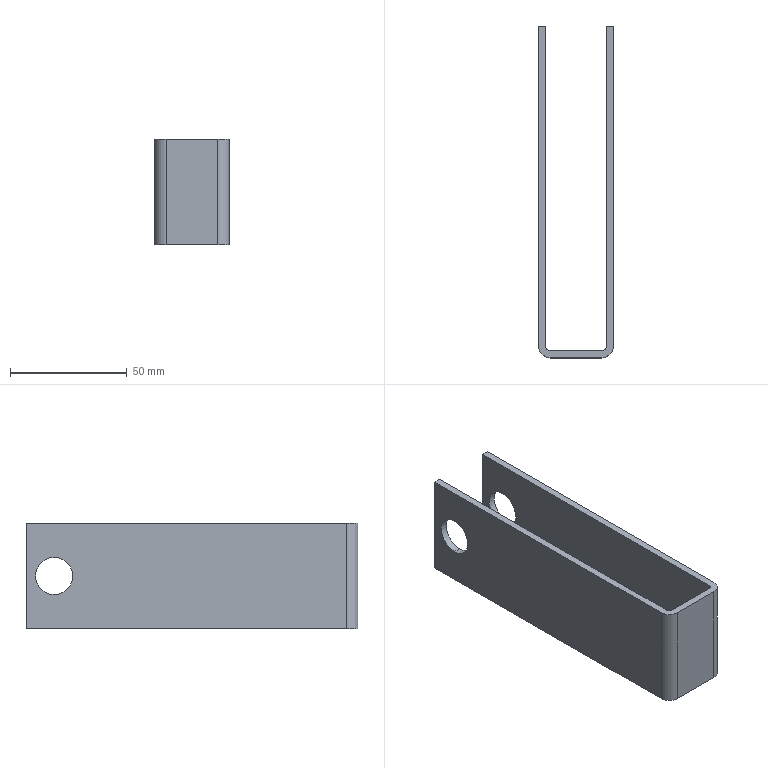Part | SolidWorks | features Extrusion 1, ICE 1 | 1 solid | 18 faces | box 32 x 142 x 45 mm | volume 40238 mm3 | plane 10 | cylinder 8 | commonest cylinder face diameters 16 x4 4 x2 10 x2
STEP:
#1=CARTESIAN_POINT('',(29.,-12.,30.5));
#2=VERTEX_POINT('',#1);
#3=CARTESIAN_POINT('',(29.,-12.,14.5));
#4=VERTEX_POINT('',#3);
#5=CARTESIAN_POINT('',(29.,-12.,22.5));
#6=DIRECTION('',(1.,0.,0.));
#7=DIRECTION('',(0.,1.,0.));
#8=AXIS2_PLACEMENT_3D('',#5,#6,#7);
#9=CIRCLE('',#8,8.);
#10=EDGE_CURVE('',#2,#4,#9,.T.);
#11=ORIENTED_EDGE('',*,*,#10,.F.);
#12=CARTESIAN_POINT('',(32.,-12.,30.5));
#13=VERTEX_POINT('',#12);
#14=CARTESIAN_POINT('',(0.,-12.,30.5));
#15=DIRECTION('',(1.,0.,0.));
#16=VECTOR('',#15,1000.);
#17=LINE('',#14,#16);
#18=EDGE_CURVE('',#2,#13,#17,.T.);
#19=ORIENTED_EDGE('',*,*,#18,.T.);
#20=CARTESIAN_POINT('',(32.,-12.,14.5));
#21=VERTEX_POINT('',#20);
#22=CARTESIAN_POINT('',(32.,-12.,22.5));
#23=DIRECTION('',(1.,0.,0.));
#24=DIRECTION('',(0.,0.,-1.));
#25=AXIS2_PLACEMENT_3D('',#22,#23,#24);
#26=CIRCLE('',#25,8.);
#27=EDGE_CURVE('',#13,#21,#26,.T.);
#28=ORIENTED_EDGE('',*,*,#27,.T.);
#29=CARTESIAN_POINT('',(0.,-12.,14.5));
#30=DIRECTION('',(1.,0.,0.));
#31=VECTOR('',#30,1000.);
#32=LINE('',#29,#31);
#33=EDGE_CURVE('',#4,#21,#32,.T.);
#34=ORIENTED_EDGE('',*,*,#33,.F.);
#35=EDGE_LOOP('',(#11,#19,#28,#34));
#36=FACE_OUTER_BOUND('',#35,.T.);
#37=CARTESIAN_POINT('',(0.,-12.,22.5));
#38=DIRECTION('',(1.,0.,0.));
#39=DIRECTION('',(0.,0.,-1.));
#40=AXIS2_PLACEMENT_3D('',#37,#38,#39);
#41=CYLINDRICAL_SURFACE('',#40,8.);
#42=ADVANCED_FACE('',(#36),#41,.F.);
#43=CARTESIAN_POINT('',(0.,-12.,30.5));
#44=VERTEX_POINT('',#43);
#45=CARTESIAN_POINT('',(0.,-12.,14.5));
#46=VERTEX_POINT('',#45);
#47=CARTESIAN_POINT('',(0.,-12.,22.5));
#48=DIRECTION('',(1.,0.,0.));
#49=DIRECTION('',(0.,0.,-1.));
#50=AXIS2_PLACEMENT_3D('',#47,#48,#49);
#51=CIRCLE('',#50,8.);
#52=EDGE_CURVE('',#44,#46,#51,.T.);
#53=ORIENTED_EDGE('',*,*,#52,.F.);
#54=CARTESIAN_POINT('',(3.,-12.,30.5));
#55=VERTEX_POINT('',#54);
#56=CARTESIAN_POINT('',(0.,-12.,30.5));
#57=DIRECTION('',(1.,0.,0.));
#58=VECTOR('',#57,1000.);
#59=LINE('',#56,#58);
#60=EDGE_CURVE('',#44,#55,#59,.T.);
#61=ORIENTED_EDGE('',*,*,#60,.T.);
#62=CARTESIAN_POINT('',(3.,-12.,14.5));
#63=VERTEX_POINT('',#62);
#64=CARTESIAN_POINT('',(3.,-12.,22.5));
#65=DIRECTION('',(-1.,0.,0.));
#66=DIRECTION('',(0.,-1.,0.));
#67=AXIS2_PLACEMENT_3D('',#64,#65,#66);
#68=CIRCLE('',#67,8.);
#69=EDGE_CURVE('',#63,#55,#68,.T.);
#70=ORIENTED_EDGE('',*,*,#69,.F.);
#71=CARTESIAN_POINT('',(0.,-12.,14.5));
#72=DIRECTION('',(1.,0.,0.));
#73=VECTOR('',#72,1000.);
#74=LINE('',#71,#73);
#75=EDGE_CURVE('',#46,#63,#74,.T.);
#76=ORIENTED_EDGE('',*,*,#75,.F.);
#77=EDGE_LOOP('',(#53,#61,#70,#76));
#78=FACE_OUTER_BOUND('',#77,.T.);
#79=CARTESIAN_POINT('',(0.,-12.,22.5));
#80=DIRECTION('',(1.,0.,0.));
#81=DIRECTION('',(0.,0.,-1.));
#82=AXIS2_PLACEMENT_3D('',#79,#80,#81);
#83=CYLINDRICAL_SURFACE('',#82,8.);
#84=ADVANCED_FACE('',(#78),#83,.F.);
#85=CARTESIAN_POINT('',(3.,0.,0.));
#86=VERTEX_POINT('',#85);
#87=CARTESIAN_POINT('',(0.,0.,0.));
#88=VERTEX_POINT('',#87);
#89=CARTESIAN_POINT('',(3.,0.,0.));
#90=DIRECTION('',(-1.,0.,0.));
#91=VECTOR('',#90,1000.);
#92=LINE('',#89,#91);
#93=EDGE_CURVE('',#86,#88,#92,.T.);
#94=ORIENTED_EDGE('',*,*,#93,.T.);
#95=CARTESIAN_POINT('',(0.,0.,45.));
#96=VERTEX_POINT('',#95);
#97=CARTESIAN_POINT('',(0.,0.,45.));
#98=DIRECTION('',(0.,0.,-1.));
#99=VECTOR('',#98,1000.);
#100=LINE('',#97,#99);
#101=EDGE_CURVE('',#96,#88,#100,.T.);
#102=ORIENTED_EDGE('',*,*,#101,.F.);
#103=CARTESIAN_POINT('',(3.,0.,45.));
#104=VERTEX_POINT('',#103);
#105=CARTESIAN_POINT('',(3.,0.,45.));
#106=DIRECTION('',(-1.,0.,0.));
#107=VECTOR('',#106,1000.);
#108=LINE('',#105,#107);
#109=EDGE_CURVE('',#104,#96,#108,.T.);
#110=ORIENTED_EDGE('',*,*,#109,.F.);
#111=CARTESIAN_POINT('',(3.,0.,45.));
#112=DIRECTION('',(0.,0.,-1.));
#113=VECTOR('',#112,1000.);
#114=LINE('',#111,#113);
#115=EDGE_CURVE('',#104,#86,#114,.T.);
#116=ORIENTED_EDGE('',*,*,#115,.T.);
#117=EDGE_LOOP('',(#94,#102,#110,#116));
#118=FACE_OUTER_BOUND('',#117,.T.);
#119=CARTESIAN_POINT('',(3.,0.,45.));
#120=DIRECTION('',(0.,-1.,0.));
#121=DIRECTION('',(0.,0.,-1.));
#122=AXIS2_PLACEMENT_3D('',#119,#120,#121);
#123=PLANE('',#122);
#124=ADVANCED_FACE('',(#118),#123,.F.);
#125=CARTESIAN_POINT('',(0.,-12.,22.5));
#126=DIRECTION('',(1.,0.,0.));
#127=DIRECTION('',(0.,0.,-1.));
#128=AXIS2_PLACEMENT_3D('',#125,#126,#127);
#129=CIRCLE('',#128,8.);
#130=EDGE_CURVE('',#46,#44,#129,.T.);
#131=ORIENTED_EDGE('',*,*,#130,.T.);
#132=ORIENTED_EDGE('',*,*,#52,.T.);
#133=EDGE_LOOP('',(#131,#132));
#134=FACE_BOUND('',#133,.T.);
#135=CARTESIAN_POINT('',(0.,-137.,0.));
#136=VERTEX_POINT('',#135);
#137=CARTESIAN_POINT('',(0.,0.,0.));
#138=DIRECTION('',(0.,-1.,0.));
#139=VECTOR('',#138,1000.);
#140=LINE('',#137,#139);
#141=EDGE_CURVE('',#88,#136,#140,.T.);
#142=ORIENTED_EDGE('',*,*,#141,.T.);
#143=CARTESIAN_POINT('',(0.,-137.,45.));
#144=VERTEX_POINT('',#143);
#145=CARTESIAN_POINT('',(0.,-137.,45.));
#146=DIRECTION('',(0.,0.,-1.));
#147=VECTOR('',#146,1000.);
#148=LINE('',#145,#147);
#149=EDGE_CURVE('',#144,#136,#148,.T.);
#150=ORIENTED_EDGE('',*,*,#149,.F.);
#151=CARTESIAN_POINT('',(0.,0.,45.));
#152=DIRECTION('',(0.,-1.,0.));
#153=VECTOR('',#152,1000.);
#154=LINE('',#151,#153);
#155=EDGE_CURVE('',#96,#144,#154,.T.);
#156=ORIENTED_EDGE('',*,*,#155,.F.);
#157=ORIENTED_EDGE('',*,*,#101,.T.);
#158=EDGE_LOOP('',(#142,#150,#156,#157));
#159=FACE_OUTER_BOUND('',#158,.T.);
#160=CARTESIAN_POINT('',(0.,0.,45.));
#161=DIRECTION('',(1.,0.,0.));
#162=DIRECTION('',(0.,1.,0.));
#163=AXIS2_PLACEMENT_3D('',#160,#161,#162);
#164=PLANE('',#163);
#165=ADVANCED_FACE('',(#134,#159),#164,.F.);
#166=CARTESIAN_POINT('',(5.,-142.,0.));
#167=VERTEX_POINT('',#166);
#168=CARTESIAN_POINT('',(5.,-137.,0.));
#169=DIRECTION('',(0.,0.,1.));
#170=DIRECTION('',(1.,0.,0.));
#171=AXIS2_PLACEMENT_3D('',#168,#169,#170);
#172=CIRCLE('',#171,5.);
#173=EDGE_CURVE('',#136,#167,#172,.T.);
#174=ORIENTED_EDGE('',*,*,#173,.T.);
#175=CARTESIAN_POINT('',(5.,-142.,45.));
#176=VERTEX_POINT('',#175);
#177=CARTESIAN_POINT('',(5.,-142.,45.));
#178=DIRECTION('',(0.,0.,-1.));
#179=VECTOR('',#178,1000.);
#180=LINE('',#177,#179);
#181=EDGE_CURVE('',#176,#167,#180,.T.);
#182=ORIENTED_EDGE('',*,*,#181,.F.);
#183=CARTESIAN_POINT('',(5.,-137.,45.));
#184=DIRECTION('',(0.,0.,1.));
#185=DIRECTION('',(1.,0.,0.));
#186=AXIS2_PLACEMENT_3D('',#183,#184,#185);
#187=CIRCLE('',#186,5.);
#188=EDGE_CURVE('',#144,#176,#187,.T.);
#189=ORIENTED_EDGE('',*,*,#188,.F.);
#190=ORIENTED_EDGE('',*,*,#149,.T.);
#191=EDGE_LOOP('',(#174,#182,#189,#190));
#192=FACE_OUTER_BOUND('',#191,.T.);
#193=CARTESIAN_POINT('',(5.,-137.,45.));
#194=DIRECTION('',(0.,0.,-1.));
#195=DIRECTION('',(-1.,0.,0.));
#196=AXIS2_PLACEMENT_3D('',#193,#194,#195);
#197=CYLINDRICAL_SURFACE('',#196,5.);
#198=ADVANCED_FACE('',(#192),#197,.T.);
#199=CARTESIAN_POINT('',(27.,-142.,0.));
#200=VERTEX_POINT('',#199);
#201=CARTESIAN_POINT('',(5.,-142.,0.));
#202=DIRECTION('',(1.,0.,0.));
#203=VECTOR('',#202,1000.);
#204=LINE('',#201,#203);
#205=EDGE_CURVE('',#167,#200,#204,.T.);
#206=ORIENTED_EDGE('',*,*,#205,.T.);
#207=CARTESIAN_POINT('',(27.,-142.,45.));
#208=VERTEX_POINT('',#207);
#209=CARTESIAN_POINT('',(27.,-142.,45.));
#210=DIRECTION('',(0.,0.,-1.));
#211=VECTOR('',#210,1000.);
#212=LINE('',#209,#211);
#213=EDGE_CURVE('',#208,#200,#212,.T.);
#214=ORIENTED_EDGE('',*,*,#213,.F.);
#215=CARTESIAN_POINT('',(5.,-142.,45.));
#216=DIRECTION('',(1.,0.,0.));
#217=VECTOR('',#216,1000.);
#218=LINE('',#215,#217);
#219=EDGE_CURVE('',#176,#208,#218,.T.);
#220=ORIENTED_EDGE('',*,*,#219,.F.);
#221=ORIENTED_EDGE('',*,*,#181,.T.);
#222=EDGE_LOOP('',(#206,#214,#220,#221));
#223=FACE_OUTER_BOUND('',#222,.T.);
#224=CARTESIAN_POINT('',(5.,-142.,45.));
#225=DIRECTION('',(0.,1.,0.));
#226=DIRECTION('',(0.,0.,1.));
#227=AXIS2_PLACEMENT_3D('',#224,#225,#226);
#228=PLANE('',#227);
#229=ADVANCED_FACE('',(#223),#228,.F.);
#230=CARTESIAN_POINT('',(32.,-137.,0.));
#231=VERTEX_POINT('',#230);
#232=CARTESIAN_POINT('',(27.,-137.,0.));
#233=DIRECTION('',(0.,0.,1.));
#234=DIRECTION('',(1.,0.,0.));
#235=AXIS2_PLACEMENT_3D('',#232,#233,#234);
#236=CIRCLE('',#235,5.);
#237=EDGE_CURVE('',#200,#231,#236,.T.);
#238=ORIENTED_EDGE('',*,*,#237,.T.);
#239=CARTESIAN_POINT('',(32.,-137.,45.));
#240=VERTEX_POINT('',#239);
#241=CARTESIAN_POINT('',(32.,-137.,45.));
#242=DIRECTION('',(0.,0.,-1.));
#243=VECTOR('',#242,1000.);
#244=LINE('',#241,#243);
#245=EDGE_CURVE('',#240,#231,#244,.T.);
#246=ORIENTED_EDGE('',*,*,#245,.F.);
#247=CARTESIAN_POINT('',(27.,-137.,45.));
#248=DIRECTION('',(0.,0.,1.));
#249=DIRECTION('',(1.,0.,0.));
#250=AXIS2_PLACEMENT_3D('',#247,#248,#249);
#251=CIRCLE('',#250,5.);
#252=EDGE_CURVE('',#208,#240,#251,.T.);
#253=ORIENTED_EDGE('',*,*,#252,.F.);
#254=ORIENTED_EDGE('',*,*,#213,.T.);
#255=EDGE_LOOP('',(#238,#246,#253,#254));
#256=FACE_OUTER_BOUND('',#255,.T.);
#257=CARTESIAN_POINT('',(27.,-137.,45.));
#258=DIRECTION('',(0.,0.,-1.));
#259=DIRECTION('',(-1.,0.,0.));
#260=AXIS2_PLACEMENT_3D('',#257,#258,#259);
#261=CYLINDRICAL_SURFACE('',#260,5.);
#262=ADVANCED_FACE('',(#256),#261,.T.);
#263=CARTESIAN_POINT('',(32.,-12.,22.5));
#264=DIRECTION('',(1.,0.,0.));
#265=DIRECTION('',(0.,0.,-1.));
#266=AXIS2_PLACEMENT_3D('',#263,#264,#265);
#267=CIRCLE('',#266,8.);
#268=EDGE_CURVE('',#21,#13,#267,.T.);
#269=ORIENTED_EDGE('',*,*,#268,.F.);
#270=ORIENTED_EDGE('',*,*,#27,.F.);
#271=EDGE_LOOP('',(#269,#270));
#272=FACE_BOUND('',#271,.T.);
#273=CARTESIAN_POINT('',(32.,0.,0.));
#274=VERTEX_POINT('',#273);
#275=CARTESIAN_POINT('',(32.,-137.,0.));
#276=DIRECTION('',(0.,1.,0.));
#277=VECTOR('',#276,1000.);
#278=LINE('',#275,#277);
#279=EDGE_CURVE('',#231,#274,#278,.T.);
#280=ORIENTED_EDGE('',*,*,#279,.T.);
#281=CARTESIAN_POINT('',(32.,0.,45.));
#282=VERTEX_POINT('',#281);
#283=CARTESIAN_POINT('',(32.,0.,45.));
#284=DIRECTION('',(0.,0.,-1.));
#285=VECTOR('',#284,1000.);
#286=LINE('',#283,#285);
#287=EDGE_CURVE('',#282,#274,#286,.T.);
#288=ORIENTED_EDGE('',*,*,#287,.F.);
#289=CARTESIAN_POINT('',(32.,-137.,45.));
#290=DIRECTION('',(0.,1.,0.));
#291=VECTOR('',#290,1000.);
#292=LINE('',#289,#291);
#293=EDGE_CURVE('',#240,#282,#292,.T.);
#294=ORIENTED_EDGE('',*,*,#293,.F.);
#295=ORIENTED_EDGE('',*,*,#245,.T.);
#296=EDGE_LOOP('',(#280,#288,#294,#295));
#297=FACE_OUTER_BOUND('',#296,.T.);
#298=CARTESIAN_POINT('',(32.,-137.,45.));
#299=DIRECTION('',(-1.,0.,0.));
#300=DIRECTION('',(0.,-1.,0.));
#301=AXIS2_PLACEMENT_3D('',#298,#299,#300);
#302=PLANE('',#301);
#303=ADVANCED_FACE('',(#272,#297),#302,.F.);
#304=CARTESIAN_POINT('',(29.,0.,0.));
#305=VERTEX_POINT('',#304);
#306=CARTESIAN_POINT('',(29.,0.,0.));
#307=DIRECTION('',(-1.,0.,0.));
#308=VECTOR('',#307,1000.);
#309=LINE('',#306,#308);
#310=EDGE_CURVE('',#274,#305,#309,.T.);
#311=ORIENTED_EDGE('',*,*,#310,.T.);
#312=CARTESIAN_POINT('',(29.,0.,45.));
#313=VERTEX_POINT('',#312);
#314=CARTESIAN_POINT('',(29.,0.,45.));
#315=DIRECTION('',(0.,0.,-1.));
#316=VECTOR('',#315,1000.);
#317=LINE('',#314,#316);
#318=EDGE_CURVE('',#313,#305,#317,.T.);
#319=ORIENTED_EDGE('',*,*,#318,.F.);
#320=CARTESIAN_POINT('',(29.,0.,45.));
#321=DIRECTION('',(-1.,0.,0.));
#322=VECTOR('',#321,1000.);
#323=LINE('',#320,#322);
#324=EDGE_CURVE('',#282,#313,#323,.T.);
#325=ORIENTED_EDGE('',*,*,#324,.F.);
#326=ORIENTED_EDGE('',*,*,#287,.T.);
#327=EDGE_LOOP('',(#311,#319,#325,#326));
#328=FACE_OUTER_BOUND('',#327,.T.);
#329=CARTESIAN_POINT('',(29.,0.,45.));
#330=DIRECTION('',(0.,-1.,0.));
#331=DIRECTION('',(1.,0.,0.));
#332=AXIS2_PLACEMENT_3D('',#329,#330,#331);
#333=PLANE('',#332);
#334=ADVANCED_FACE('',(#328),#333,.F.);
#335=CARTESIAN_POINT('',(29.,-12.,22.5));
#336=DIRECTION('',(1.,0.,0.));
#337=DIRECTION('',(0.,1.,0.));
#338=AXIS2_PLACEMENT_3D('',#335,#336,#337);
#339=CIRCLE('',#338,8.);
#340=EDGE_CURVE('',#4,#2,#339,.T.);
#341=ORIENTED_EDGE('',*,*,#340,.T.);
#342=ORIENTED_EDGE('',*,*,#10,.T.);
#343=EDGE_LOOP('',(#341,#342));
#344=FACE_BOUND('',#343,.T.);
#345=CARTESIAN_POINT('',(29.,-137.,0.));
#346=VERTEX_POINT('',#345);
#347=CARTESIAN_POINT('',(29.,-137.,0.));
#348=DIRECTION('',(0.,-1.,0.));
#349=VECTOR('',#348,1000.);
#350=LINE('',#347,#349);
#351=EDGE_CURVE('',#305,#346,#350,.T.);
#352=ORIENTED_EDGE('',*,*,#351,.T.);
#353=CARTESIAN_POINT('',(29.,-137.,45.));
#354=VERTEX_POINT('',#353);
#355=CARTESIAN_POINT('',(29.,-137.,45.));
#356=DIRECTION('',(0.,0.,-1.));
#357=VECTOR('',#356,1000.);
#358=LINE('',#355,#357);
#359=EDGE_CURVE('',#354,#346,#358,.T.);
#360=ORIENTED_EDGE('',*,*,#359,.F.);
#361=CARTESIAN_POINT('',(29.,-137.,45.));
#362=DIRECTION('',(0.,-1.,0.));
#363=VECTOR('',#362,1000.);
#364=LINE('',#361,#363);
#365=EDGE_CURVE('',#313,#354,#364,.T.);
#366=ORIENTED_EDGE('',*,*,#365,.F.);
#367=ORIENTED_EDGE('',*,*,#318,.T.);
#368=EDGE_LOOP('',(#352,#360,#366,#367));
#369=FACE_OUTER_BOUND('',#368,.T.);
#370=CARTESIAN_POINT('',(29.,-137.,45.));
#371=DIRECTION('',(1.,0.,0.));
#372=DIRECTION('',(0.,1.,0.));
#373=AXIS2_PLACEMENT_3D('',#370,#371,#372);
#374=PLANE('',#373);
#375=ADVANCED_FACE('',(#344,#369),#374,.F.);
#376=CARTESIAN_POINT('',(27.,-139.,0.));
#377=VERTEX_POINT('',#376);
#378=CARTESIAN_POINT('',(27.,-137.,0.));
#379=DIRECTION('',(0.,0.,-1.));
#380=DIRECTION('',(1.,0.,0.));
#381=AXIS2_PLACEMENT_3D('',#378,#379,#380);
#382=CIRCLE('',#381,2.);
#383=EDGE_CURVE('',#346,#377,#382,.T.);
#384=ORIENTED_EDGE('',*,*,#383,.T.);
#385=CARTESIAN_POINT('',(27.,-139.,45.));
#386=VERTEX_POINT('',#385);
#387=CARTESIAN_POINT('',(27.,-139.,45.));
#388=DIRECTION('',(0.,0.,-1.));
#389=VECTOR('',#388,1000.);
#390=LINE('',#387,#389);
#391=EDGE_CURVE('',#386,#377,#390,.T.);
#392=ORIENTED_EDGE('',*,*,#391,.F.);
#393=CARTESIAN_POINT('',(27.,-137.,45.));
#394=DIRECTION('',(0.,0.,-1.));
#395=DIRECTION('',(1.,0.,0.));
#396=AXIS2_PLACEMENT_3D('',#393,#394,#395);
#397=CIRCLE('',#396,2.);
#398=EDGE_CURVE('',#354,#386,#397,.T.);
#399=ORIENTED_EDGE('',*,*,#398,.F.);
#400=ORIENTED_EDGE('',*,*,#359,.T.);
#401=EDGE_LOOP('',(#384,#392,#399,#400));
#402=FACE_OUTER_BOUND('',#401,.T.);
#403=CARTESIAN_POINT('',(27.,-137.,45.));
#404=DIRECTION('',(0.,0.,-1.));
#405=DIRECTION('',(-1.,0.,0.));
#406=AXIS2_PLACEMENT_3D('',#403,#404,#405);
#407=CYLINDRICAL_SURFACE('',#406,2.);
#408=ADVANCED_FACE('',(#402),#407,.F.);
#409=CARTESIAN_POINT('',(5.,-139.,0.));
#410=VERTEX_POINT('',#409);
#411=CARTESIAN_POINT('',(5.,-139.,0.));
#412=DIRECTION('',(-1.,0.,0.));
#413=VECTOR('',#412,1000.);
#414=LINE('',#411,#413);
#415=EDGE_CURVE('',#377,#410,#414,.T.);
#416=ORIENTED_EDGE('',*,*,#415,.T.);
#417=CARTESIAN_POINT('',(5.,-139.,45.));
#418=VERTEX_POINT('',#417);
#419=CARTESIAN_POINT('',(5.,-139.,45.));
#420=DIRECTION('',(0.,0.,-1.));
#421=VECTOR('',#420,1000.);
#422=LINE('',#419,#421);
#423=EDGE_CURVE('',#418,#410,#422,.T.);
#424=ORIENTED_EDGE('',*,*,#423,.F.);
#425=CARTESIAN_POINT('',(5.,-139.,45.));
#426=DIRECTION('',(-1.,0.,0.));
#427=VECTOR('',#426,1000.);
#428=LINE('',#425,#427);
#429=EDGE_CURVE('',#386,#418,#428,.T.);
#430=ORIENTED_EDGE('',*,*,#429,.F.);
#431=ORIENTED_EDGE('',*,*,#391,.T.);
#432=EDGE_LOOP('',(#416,#424,#430,#431));
#433=FACE_OUTER_BOUND('',#432,.T.);
#434=CARTESIAN_POINT('',(5.,-139.,45.));
#435=DIRECTION('',(0.,-1.,0.));
#436=DIRECTION('',(0.,0.,-1.));
#437=AXIS2_PLACEMENT_3D('',#434,#435,#436);
#438=PLANE('',#437);
#439=ADVANCED_FACE('',(#433),#438,.F.);
#440=CARTESIAN_POINT('',(3.,-137.,0.));
#441=VERTEX_POINT('',#440);
#442=CARTESIAN_POINT('',(5.,-137.,0.));
#443=DIRECTION('',(0.,0.,-1.));
#444=DIRECTION('',(1.,0.,0.));
#445=AXIS2_PLACEMENT_3D('',#442,#443,#444);
#446=CIRCLE('',#445,2.);
#447=EDGE_CURVE('',#410,#441,#446,.T.);
#448=ORIENTED_EDGE('',*,*,#447,.T.);
#449=CARTESIAN_POINT('',(3.,-137.,45.));
#450=VERTEX_POINT('',#449);
#451=CARTESIAN_POINT('',(3.,-137.,45.));
#452=DIRECTION('',(0.,0.,-1.));
#453=VECTOR('',#452,1000.);
#454=LINE('',#451,#453);
#455=EDGE_CURVE('',#450,#441,#454,.T.);
#456=ORIENTED_EDGE('',*,*,#455,.F.);
#457=CARTESIAN_POINT('',(5.,-137.,45.));
#458=DIRECTION('',(0.,0.,-1.));
#459=DIRECTION('',(1.,0.,0.));
#460=AXIS2_PLACEMENT_3D('',#457,#458,#459);
#461=CIRCLE('',#460,2.);
#462=EDGE_CURVE('',#418,#450,#461,.T.);
#463=ORIENTED_EDGE('',*,*,#462,.F.);
#464=ORIENTED_EDGE('',*,*,#423,.T.);
#465=EDGE_LOOP('',(#448,#456,#463,#464));
#466=FACE_OUTER_BOUND('',#465,.T.);
#467=CARTESIAN_POINT('',(5.,-137.,45.));
#468=DIRECTION('',(0.,0.,-1.));
#469=DIRECTION('',(-1.,0.,0.));
#470=AXIS2_PLACEMENT_3D('',#467,#468,#469);
#471=CYLINDRICAL_SURFACE('',#470,2.);
#472=ADVANCED_FACE('',(#466),#471,.F.);
#473=ORIENTED_EDGE('',*,*,#69,.T.);
#474=CARTESIAN_POINT('',(3.,-12.,22.5));
#475=DIRECTION('',(-1.,0.,0.));
#476=DIRECTION('',(0.,-1.,0.));
#477=AXIS2_PLACEMENT_3D('',#474,#475,#476);
#478=CIRCLE('',#477,8.);
#479=EDGE_CURVE('',#55,#63,#478,.T.);
#480=ORIENTED_EDGE('',*,*,#479,.T.);
#481=EDGE_LOOP('',(#473,#480));
#482=FACE_BOUND('',#481,.T.);
#483=CARTESIAN_POINT('',(3.,0.,0.));
#484=DIRECTION('',(0.,1.,0.));
#485=VECTOR('',#484,1000.);
#486=LINE('',#483,#485);
#487=EDGE_CURVE('',#441,#86,#486,.T.);
#488=ORIENTED_EDGE('',*,*,#487,.T.);
#489=ORIENTED_EDGE('',*,*,#115,.F.);
#490=CARTESIAN_POINT('',(3.,0.,45.));
#491=DIRECTION('',(0.,1.,0.));
#492=VECTOR('',#491,1000.);
#493=LINE('',#490,#492);
#494=EDGE_CURVE('',#450,#104,#493,.T.);
#495=ORIENTED_EDGE('',*,*,#494,.F.);
#496=ORIENTED_EDGE('',*,*,#455,.T.);
#497=EDGE_LOOP('',(#488,#489,#495,#496));
#498=FACE_OUTER_BOUND('',#497,.T.);
#499=CARTESIAN_POINT('',(3.,0.,45.));
#500=DIRECTION('',(-1.,0.,0.));
#501=DIRECTION('',(0.,-1.,0.));
#502=AXIS2_PLACEMENT_3D('',#499,#500,#501);
#503=PLANE('',#502);
#504=ADVANCED_FACE('',(#482,#498),#503,.F.);
#505=ORIENTED_EDGE('',*,*,#109,.T.);
#506=ORIENTED_EDGE('',*,*,#155,.T.);
#507=ORIENTED_EDGE('',*,*,#188,.T.);
#508=ORIENTED_EDGE('',*,*,#219,.T.);
#509=ORIENTED_EDGE('',*,*,#252,.T.);
#510=ORIENTED_EDGE('',*,*,#293,.T.);
#511=ORIENTED_EDGE('',*,*,#324,.T.);
#512=ORIENTED_EDGE('',*,*,#365,.T.);
#513=ORIENTED_EDGE('',*,*,#398,.T.);
#514=ORIENTED_EDGE('',*,*,#429,.T.);
#515=ORIENTED_EDGE('',*,*,#462,.T.);
#516=ORIENTED_EDGE('',*,*,#494,.T.);
#517=EDGE_LOOP('',(#505,#506,#507,#508,#509,#510,#511,#512,#513,#514,#515,#516));
#518=FACE_OUTER_BOUND('',#517,.T.);
#519=CARTESIAN_POINT('',(5.,-137.,45.));
#520=DIRECTION('',(0.,0.,1.));
#521=DIRECTION('',(1.,0.,0.));
#522=AXIS2_PLACEMENT_3D('',#519,#520,#521);
#523=PLANE('',#522);
#524=ADVANCED_FACE('',(#518),#523,.T.);
#525=ORIENTED_EDGE('',*,*,#93,.F.);
#526=ORIENTED_EDGE('',*,*,#487,.F.);
#527=ORIENTED_EDGE('',*,*,#447,.F.);
#528=ORIENTED_EDGE('',*,*,#415,.F.);
#529=ORIENTED_EDGE('',*,*,#383,.F.);
#530=ORIENTED_EDGE('',*,*,#351,.F.);
#531=ORIENTED_EDGE('',*,*,#310,.F.);
#532=ORIENTED_EDGE('',*,*,#279,.F.);
#533=ORIENTED_EDGE('',*,*,#237,.F.);
#534=ORIENTED_EDGE('',*,*,#205,.F.);
#535=ORIENTED_EDGE('',*,*,#173,.F.);
#536=ORIENTED_EDGE('',*,*,#141,.F.);
#537=EDGE_LOOP('',(#525,#526,#527,#528,#529,#530,#531,#532,#533,#534,#535,#536));
#538=FACE_OUTER_BOUND('',#537,.T.);
#539=CARTESIAN_POINT('',(5.,-137.,0.));
#540=DIRECTION('',(0.,0.,1.));
#541=DIRECTION('',(1.,0.,0.));
#542=AXIS2_PLACEMENT_3D('',#539,#540,#541);
#543=PLANE('',#542);
#544=ADVANCED_FACE('',(#538),#543,.F.);
#545=ORIENTED_EDGE('',*,*,#60,.F.);
#546=ORIENTED_EDGE('',*,*,#130,.F.);
#547=ORIENTED_EDGE('',*,*,#75,.T.);
#548=ORIENTED_EDGE('',*,*,#479,.F.);
#549=EDGE_LOOP('',(#545,#546,#547,#548));
#550=FACE_OUTER_BOUND('',#549,.T.);
#551=CARTESIAN_POINT('',(0.,-12.,22.5));
#552=DIRECTION('',(1.,0.,0.));
#553=DIRECTION('',(0.,0.,-1.));
#554=AXIS2_PLACEMENT_3D('',#551,#552,#553);
#555=CYLINDRICAL_SURFACE('',#554,8.);
#556=ADVANCED_FACE('',(#550),#555,.F.);
#557=ORIENTED_EDGE('',*,*,#18,.F.);
#558=ORIENTED_EDGE('',*,*,#340,.F.);
#559=ORIENTED_EDGE('',*,*,#33,.T.);
#560=ORIENTED_EDGE('',*,*,#268,.T.);
#561=EDGE_LOOP('',(#557,#558,#559,#560));
#562=FACE_OUTER_BOUND('',#561,.T.);
#563=CARTESIAN_POINT('',(0.,-12.,22.5));
#564=DIRECTION('',(1.,0.,0.));
#565=DIRECTION('',(0.,0.,-1.));
#566=AXIS2_PLACEMENT_3D('',#563,#564,#565);
#567=CYLINDRICAL_SURFACE('',#566,8.);
#568=ADVANCED_FACE('',(#562),#567,.F.);
#569=CLOSED_SHELL('',(#42,#84,#124,#165,#198,#229,#262,#303,#334,#375,#408,#439,#472,#504,#524,#544,#556,#568));
#570=MANIFOLD_SOLID_BREP('',#569);
#571=CARTESIAN_POINT('',(0.,0.,0.));
#572=DIRECTION('',(0.,0.,1.));
#573=DIRECTION('',(1.,0.,0.));
#574=AXIS2_PLACEMENT_3D('',#571,#572,#573);
#575=(LENGTH_UNIT()NAMED_UNIT(*)SI_UNIT(.MILLI.,.METRE.));
#576=UNCERTAINTY_MEASURE_WITH_UNIT(LENGTH_MEASURE(0.00001),#575,'','');
#577=(NAMED_UNIT(*)PLANE_ANGLE_UNIT()SI_UNIT($,.RADIAN.));
#578=(NAMED_UNIT(*)SI_UNIT($,.STERADIAN.)SOLID_ANGLE_UNIT());
#579=(GEOMETRIC_REPRESENTATION_CONTEXT(3)GLOBAL_UNCERTAINTY_ASSIGNED_CONTEXT((#576))GLOBAL_UNIT_ASSIGNED_CONTEXT((#575,#577,#578))REPRESENTATION_CONTEXT('',''));
#580=ADVANCED_BREP_SHAPE_REPRESENTATION('',(#570,#574),#579);